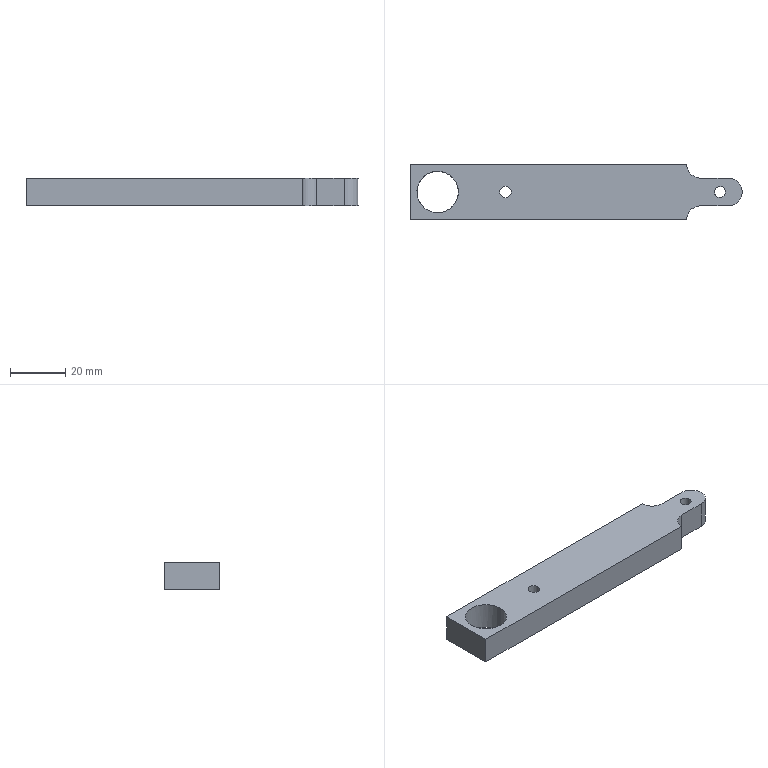Part | NX | features DATUM_CSYS 5, EXTRUDE 4, SKETCH 4, BLEND 2 | 1 solid | 13 faces | box 120 x 20 x 10 mm | volume 19969 mm3 | plane 7 | cylinder 6 | commonest cylinder face diameters 10 x3 4 x1 4.2 x1 15 x1
STEP:
#1=CARTESIAN_POINT('',(-60.,10.,0.));
#2=VERTEX_POINT('',#1);
#3=CARTESIAN_POINT('',(-60.,-10.,0.));
#4=VERTEX_POINT('',#3);
#5=CARTESIAN_POINT('',(-60.,10.,0.));
#6=DIRECTION('',(0.,-1.,0.));
#7=VECTOR('',#6,1000.);
#8=LINE('',#5,#7);
#9=EDGE_CURVE('',#2,#4,#8,.T.);
#10=ORIENTED_EDGE('',*,*,#9,.T.);
#11=CARTESIAN_POINT('',(-60.,-10.,10.));
#12=VERTEX_POINT('',#11);
#13=CARTESIAN_POINT('',(-60.,-10.,10.));
#14=DIRECTION('',(0.,0.,-1.));
#15=VECTOR('',#14,1000.);
#16=LINE('',#13,#15);
#17=EDGE_CURVE('',#12,#4,#16,.T.);
#18=ORIENTED_EDGE('',*,*,#17,.F.);
#19=CARTESIAN_POINT('',(-60.,10.,10.));
#20=VERTEX_POINT('',#19);
#21=CARTESIAN_POINT('',(-60.,10.,10.));
#22=DIRECTION('',(0.,-1.,0.));
#23=VECTOR('',#22,1000.);
#24=LINE('',#21,#23);
#25=EDGE_CURVE('',#20,#12,#24,.T.);
#26=ORIENTED_EDGE('',*,*,#25,.F.);
#27=CARTESIAN_POINT('',(-60.,10.,10.));
#28=DIRECTION('',(0.,0.,-1.));
#29=VECTOR('',#28,1000.);
#30=LINE('',#27,#29);
#31=EDGE_CURVE('',#20,#2,#30,.T.);
#32=ORIENTED_EDGE('',*,*,#31,.T.);
#33=EDGE_LOOP('',(#10,#18,#26,#32));
#34=FACE_BOUND('',#33,.T.);
#35=CARTESIAN_POINT('',(-60.,10.,10.));
#36=DIRECTION('',(1.,0.,0.));
#37=DIRECTION('',(0.,0.,-1.));
#38=AXIS2_PLACEMENT_3D('',#35,#36,#37);
#39=PLANE('',#38);
#40=ADVANCED_FACE('',(#34),#39,.F.);
#41=CARTESIAN_POINT('',(40.,-10.,0.));
#42=VERTEX_POINT('',#41);
#43=CARTESIAN_POINT('',(-60.,-10.,0.));
#44=DIRECTION('',(1.,0.,0.));
#45=VECTOR('',#44,1000.);
#46=LINE('',#43,#45);
#47=EDGE_CURVE('',#4,#42,#46,.T.);
#48=ORIENTED_EDGE('',*,*,#47,.T.);
#49=CARTESIAN_POINT('',(40.,-10.,10.));
#50=VERTEX_POINT('',#49);
#51=CARTESIAN_POINT('',(40.,-10.,10.));
#52=DIRECTION('',(0.,0.,1.));
#53=VECTOR('',#52,1000.);
#54=LINE('',#51,#53);
#55=EDGE_CURVE('',#42,#50,#54,.T.);
#56=ORIENTED_EDGE('',*,*,#55,.T.);
#57=CARTESIAN_POINT('',(-60.,-10.,10.));
#58=DIRECTION('',(1.,0.,0.));
#59=VECTOR('',#58,1000.);
#60=LINE('',#57,#59);
#61=EDGE_CURVE('',#12,#50,#60,.T.);
#62=ORIENTED_EDGE('',*,*,#61,.F.);
#63=ORIENTED_EDGE('',*,*,#17,.T.);
#64=EDGE_LOOP('',(#48,#56,#62,#63));
#65=FACE_BOUND('',#64,.T.);
#66=CARTESIAN_POINT('',(-60.,-10.,10.));
#67=DIRECTION('',(0.,1.,0.));
#68=DIRECTION('',(0.,0.,1.));
#69=AXIS2_PLACEMENT_3D('',#66,#67,#68);
#70=PLANE('',#69);
#71=ADVANCED_FACE('',(#65),#70,.F.);
#72=CARTESIAN_POINT('',(40.,10.,10.));
#73=VERTEX_POINT('',#72);
#74=CARTESIAN_POINT('',(60.,10.,10.));
#75=DIRECTION('',(-1.,0.,0.));
#76=VECTOR('',#75,1000.);
#77=LINE('',#74,#76);
#78=EDGE_CURVE('',#73,#20,#77,.T.);
#79=ORIENTED_EDGE('',*,*,#78,.F.);
#80=CARTESIAN_POINT('',(40.,10.,0.));
#81=VERTEX_POINT('',#80);
#82=CARTESIAN_POINT('',(40.,10.,10.));
#83=DIRECTION('',(0.,0.,-1.));
#84=VECTOR('',#83,1000.);
#85=LINE('',#82,#84);
#86=EDGE_CURVE('',#73,#81,#85,.T.);
#87=ORIENTED_EDGE('',*,*,#86,.T.);
#88=CARTESIAN_POINT('',(60.,10.,0.));
#89=DIRECTION('',(-1.,0.,0.));
#90=VECTOR('',#89,1000.);
#91=LINE('',#88,#90);
#92=EDGE_CURVE('',#81,#2,#91,.T.);
#93=ORIENTED_EDGE('',*,*,#92,.T.);
#94=ORIENTED_EDGE('',*,*,#31,.F.);
#95=EDGE_LOOP('',(#79,#87,#93,#94));
#96=FACE_BOUND('',#95,.T.);
#97=CARTESIAN_POINT('',(60.,10.,10.));
#98=DIRECTION('',(0.,-1.,0.));
#99=DIRECTION('',(0.,0.,-1.));
#100=AXIS2_PLACEMENT_3D('',#97,#98,#99);
#101=PLANE('',#100);
#102=ADVANCED_FACE('',(#96),#101,.F.);
#103=CARTESIAN_POINT('',(-23.4,0.,10.));
#104=VERTEX_POINT('',#103);
#105=CARTESIAN_POINT('',(-25.5,0.,10.));
#106=DIRECTION('',(0.,0.,1.));
#107=DIRECTION('',(1.,0.,0.));
#108=AXIS2_PLACEMENT_3D('',#105,#106,#107);
#109=CIRCLE('',#108,2.1);
#110=EDGE_CURVE('',#104,#104,#109,.T.);
#111=ORIENTED_EDGE('',*,*,#110,.F.);
#112=EDGE_LOOP('',(#111));
#113=FACE_BOUND('',#112,.T.);
#114=CARTESIAN_POINT('',(55.,-5.,10.));
#115=VERTEX_POINT('',#114);
#116=CARTESIAN_POINT('',(45.,-5.,10.));
#117=VERTEX_POINT('',#116);
#118=CARTESIAN_POINT('',(126.735,-5.,10.));
#119=DIRECTION('',(-1.,0.,0.));
#120=VECTOR('',#119,1000.);
#121=LINE('',#118,#120);
#122=EDGE_CURVE('',#115,#117,#121,.T.);
#123=ORIENTED_EDGE('',*,*,#122,.F.);
#124=CARTESIAN_POINT('',(55.,5.,10.));
#125=VERTEX_POINT('',#124);
#126=CARTESIAN_POINT('',(55.,0.,10.));
#127=DIRECTION('',(0.,0.,1.));
#128=DIRECTION('',(1.,0.,0.));
#129=AXIS2_PLACEMENT_3D('',#126,#127,#128);
#130=CIRCLE('',#129,5.);
#131=EDGE_CURVE('',#115,#125,#130,.T.);
#132=ORIENTED_EDGE('',*,*,#131,.T.);
#133=CARTESIAN_POINT('',(45.,5.,10.));
#134=VERTEX_POINT('',#133);
#135=CARTESIAN_POINT('',(40.,5.,10.));
#136=DIRECTION('',(1.,0.,0.));
#137=VECTOR('',#136,1000.);
#138=LINE('',#135,#137);
#139=EDGE_CURVE('',#134,#125,#138,.T.);
#140=ORIENTED_EDGE('',*,*,#139,.F.);
#141=CARTESIAN_POINT('',(45.,10.,10.));
#142=DIRECTION('',(0.,0.,1.));
#143=DIRECTION('',(1.,0.,0.));
#144=AXIS2_PLACEMENT_3D('',#141,#142,#143);
#145=CIRCLE('',#144,5.);
#146=EDGE_CURVE('',#134,#73,#145,.F.);
#147=ORIENTED_EDGE('',*,*,#146,.T.);
#148=ORIENTED_EDGE('',*,*,#78,.T.);
#149=ORIENTED_EDGE('',*,*,#25,.T.);
#150=ORIENTED_EDGE('',*,*,#61,.T.);
#151=CARTESIAN_POINT('',(45.,-10.,10.));
#152=DIRECTION('',(0.,0.,1.));
#153=DIRECTION('',(1.,0.,0.));
#154=AXIS2_PLACEMENT_3D('',#151,#152,#153);
#155=CIRCLE('',#154,5.);
#156=EDGE_CURVE('',#50,#117,#155,.F.);
#157=ORIENTED_EDGE('',*,*,#156,.T.);
#158=EDGE_LOOP('',(#123,#132,#140,#147,#148,#149,#150,#157));
#159=FACE_BOUND('',#158,.T.);
#160=CARTESIAN_POINT('',(52.,2.,10.));
#161=VERTEX_POINT('',#160);
#162=CARTESIAN_POINT('',(52.,0.,10.));
#163=DIRECTION('',(0.,0.,1.));
#164=DIRECTION('',(0.,1.,0.));
#165=AXIS2_PLACEMENT_3D('',#162,#163,#164);
#166=CIRCLE('',#165,2.);
#167=EDGE_CURVE('',#161,#161,#166,.T.);
#168=ORIENTED_EDGE('',*,*,#167,.F.);
#169=EDGE_LOOP('',(#168));
#170=FACE_BOUND('',#169,.T.);
#171=CARTESIAN_POINT('',(-50.,7.5,10.));
#172=VERTEX_POINT('',#171);
#173=CARTESIAN_POINT('',(-50.,0.,10.));
#174=DIRECTION('',(0.,0.,1.));
#175=DIRECTION('',(0.,1.,0.));
#176=AXIS2_PLACEMENT_3D('',#173,#174,#175);
#177=CIRCLE('',#176,7.5);
#178=EDGE_CURVE('',#172,#172,#177,.T.);
#179=ORIENTED_EDGE('',*,*,#178,.F.);
#180=EDGE_LOOP('',(#179));
#181=FACE_BOUND('',#180,.T.);
#182=CARTESIAN_POINT('',(0.,0.,10.));
#183=DIRECTION('',(0.,0.,1.));
#184=DIRECTION('',(1.,0.,0.));
#185=AXIS2_PLACEMENT_3D('',#182,#183,#184);
#186=PLANE('',#185);
#187=ADVANCED_FACE('',(#113,#159,#170,#181),#186,.T.);
#188=CARTESIAN_POINT('',(-23.4,0.,0.));
#189=VERTEX_POINT('',#188);
#190=CARTESIAN_POINT('',(-25.5,0.,0.));
#191=DIRECTION('',(0.,0.,1.));
#192=DIRECTION('',(1.,0.,0.));
#193=AXIS2_PLACEMENT_3D('',#190,#191,#192);
#194=CIRCLE('',#193,2.1);
#195=EDGE_CURVE('',#189,#189,#194,.T.);
#196=ORIENTED_EDGE('',*,*,#195,.T.);
#197=EDGE_LOOP('',(#196));
#198=FACE_BOUND('',#197,.T.);
#199=CARTESIAN_POINT('',(54.,0.,0.));
#200=VERTEX_POINT('',#199);
#201=CARTESIAN_POINT('',(52.,0.,0.));
#202=DIRECTION('',(0.,0.,1.));
#203=DIRECTION('',(1.,0.,0.));
#204=AXIS2_PLACEMENT_3D('',#201,#202,#203);
#205=CIRCLE('',#204,2.);
#206=EDGE_CURVE('',#200,#200,#205,.T.);
#207=ORIENTED_EDGE('',*,*,#206,.T.);
#208=EDGE_LOOP('',(#207));
#209=FACE_BOUND('',#208,.T.);
#210=CARTESIAN_POINT('',(-42.5,0.,0.));
#211=VERTEX_POINT('',#210);
#212=CARTESIAN_POINT('',(-50.,0.,0.));
#213=DIRECTION('',(0.,0.,1.));
#214=DIRECTION('',(1.,0.,0.));
#215=AXIS2_PLACEMENT_3D('',#212,#213,#214);
#216=CIRCLE('',#215,7.5);
#217=EDGE_CURVE('',#211,#211,#216,.T.);
#218=ORIENTED_EDGE('',*,*,#217,.T.);
#219=EDGE_LOOP('',(#218));
#220=FACE_BOUND('',#219,.T.);
#221=CARTESIAN_POINT('',(55.,5.,0.));
#222=VERTEX_POINT('',#221);
#223=CARTESIAN_POINT('',(55.,-5.,0.));
#224=VERTEX_POINT('',#223);
#225=CARTESIAN_POINT('',(55.,0.,0.));
#226=DIRECTION('',(0.,0.,1.));
#227=DIRECTION('',(1.,0.,0.));
#228=AXIS2_PLACEMENT_3D('',#225,#226,#227);
#229=CIRCLE('',#228,5.);
#230=EDGE_CURVE('',#222,#224,#229,.F.);
#231=ORIENTED_EDGE('',*,*,#230,.T.);
#232=CARTESIAN_POINT('',(45.,-5.,0.));
#233=VERTEX_POINT('',#232);
#234=CARTESIAN_POINT('',(0.,-5.,0.));
#235=DIRECTION('',(-1.,0.,0.));
#236=VECTOR('',#235,1000.);
#237=LINE('',#234,#236);
#238=EDGE_CURVE('',#224,#233,#237,.T.);
#239=ORIENTED_EDGE('',*,*,#238,.T.);
#240=CARTESIAN_POINT('',(45.,-10.,0.));
#241=DIRECTION('',(0.,0.,1.));
#242=DIRECTION('',(1.,0.,0.));
#243=AXIS2_PLACEMENT_3D('',#240,#241,#242);
#244=CIRCLE('',#243,5.);
#245=EDGE_CURVE('',#233,#42,#244,.T.);
#246=ORIENTED_EDGE('',*,*,#245,.T.);
#247=ORIENTED_EDGE('',*,*,#47,.F.);
#248=ORIENTED_EDGE('',*,*,#9,.F.);
#249=ORIENTED_EDGE('',*,*,#92,.F.);
#250=CARTESIAN_POINT('',(45.,5.,0.));
#251=VERTEX_POINT('',#250);
#252=CARTESIAN_POINT('',(45.,10.,0.));
#253=DIRECTION('',(0.,0.,1.));
#254=DIRECTION('',(1.,0.,0.));
#255=AXIS2_PLACEMENT_3D('',#252,#253,#254);
#256=CIRCLE('',#255,5.);
#257=EDGE_CURVE('',#81,#251,#256,.T.);
#258=ORIENTED_EDGE('',*,*,#257,.T.);
#259=CARTESIAN_POINT('',(0.,5.,0.));
#260=DIRECTION('',(1.,0.,0.));
#261=VECTOR('',#260,1000.);
#262=LINE('',#259,#261);
#263=EDGE_CURVE('',#251,#222,#262,.T.);
#264=ORIENTED_EDGE('',*,*,#263,.T.);
#265=EDGE_LOOP('',(#231,#239,#246,#247,#248,#249,#258,#264));
#266=FACE_BOUND('',#265,.T.);
#267=CARTESIAN_POINT('',(0.,0.,0.));
#268=DIRECTION('',(0.,0.,1.));
#269=DIRECTION('',(1.,0.,0.));
#270=AXIS2_PLACEMENT_3D('',#267,#268,#269);
#271=PLANE('',#270);
#272=ADVANCED_FACE('',(#198,#209,#220,#266),#271,.F.);
#273=ORIENTED_EDGE('',*,*,#178,.T.);
#274=EDGE_LOOP('',(#273));
#275=FACE_BOUND('',#274,.T.);
#276=ORIENTED_EDGE('',*,*,#217,.F.);
#277=EDGE_LOOP('',(#276));
#278=FACE_BOUND('',#277,.T.);
#279=CARTESIAN_POINT('',(-50.,0.,-5.));
#280=DIRECTION('',(0.,0.,1.));
#281=DIRECTION('',(1.,0.,0.));
#282=AXIS2_PLACEMENT_3D('',#279,#280,#281);
#283=CYLINDRICAL_SURFACE('',#282,7.5);
#284=ADVANCED_FACE('',(#275,#278),#283,.F.);
#285=ORIENTED_EDGE('',*,*,#167,.T.);
#286=EDGE_LOOP('',(#285));
#287=FACE_BOUND('',#286,.T.);
#288=ORIENTED_EDGE('',*,*,#206,.F.);
#289=EDGE_LOOP('',(#288));
#290=FACE_BOUND('',#289,.T.);
#291=CARTESIAN_POINT('',(52.,0.,-5.));
#292=DIRECTION('',(0.,0.,1.));
#293=DIRECTION('',(1.,0.,0.));
#294=AXIS2_PLACEMENT_3D('',#291,#292,#293);
#295=CYLINDRICAL_SURFACE('',#294,2.);
#296=ADVANCED_FACE('',(#287,#290),#295,.F.);
#297=ORIENTED_EDGE('',*,*,#238,.F.);
#298=CARTESIAN_POINT('',(55.,-5.,-10.));
#299=DIRECTION('',(0.,0.,-1.));
#300=VECTOR('',#299,1000.);
#301=LINE('',#298,#300);
#302=EDGE_CURVE('',#224,#115,#301,.F.);
#303=ORIENTED_EDGE('',*,*,#302,.T.);
#304=ORIENTED_EDGE('',*,*,#122,.T.);
#305=CARTESIAN_POINT('',(45.,-5.,0.));
#306=DIRECTION('',(0.,0.,-1.));
#307=VECTOR('',#306,1000.);
#308=LINE('',#305,#307);
#309=EDGE_CURVE('',#117,#233,#308,.T.);
#310=ORIENTED_EDGE('',*,*,#309,.T.);
#311=EDGE_LOOP('',(#297,#303,#304,#310));
#312=FACE_BOUND('',#311,.T.);
#313=CARTESIAN_POINT('',(126.735,-5.,-10.));
#314=DIRECTION('',(0.,1.,0.));
#315=DIRECTION('',(-1.,0.,0.));
#316=AXIS2_PLACEMENT_3D('',#313,#314,#315);
#317=PLANE('',#316);
#318=ADVANCED_FACE('',(#312),#317,.F.);
#319=ORIENTED_EDGE('',*,*,#139,.T.);
#320=CARTESIAN_POINT('',(55.,5.,-10.));
#321=DIRECTION('',(0.,0.,1.));
#322=VECTOR('',#321,1000.);
#323=LINE('',#320,#322);
#324=EDGE_CURVE('',#125,#222,#323,.F.);
#325=ORIENTED_EDGE('',*,*,#324,.T.);
#326=ORIENTED_EDGE('',*,*,#263,.F.);
#327=CARTESIAN_POINT('',(45.,5.,10.));
#328=DIRECTION('',(0.,0.,-1.));
#329=VECTOR('',#328,1000.);
#330=LINE('',#327,#329);
#331=EDGE_CURVE('',#251,#134,#330,.F.);
#332=ORIENTED_EDGE('',*,*,#331,.T.);
#333=EDGE_LOOP('',(#319,#325,#326,#332));
#334=FACE_BOUND('',#333,.T.);
#335=CARTESIAN_POINT('',(40.,5.,-10.));
#336=DIRECTION('',(0.,-1.,0.));
#337=DIRECTION('',(1.,0.,0.));
#338=AXIS2_PLACEMENT_3D('',#335,#336,#337);
#339=PLANE('',#338);
#340=ADVANCED_FACE('',(#334),#339,.F.);
#341=ORIENTED_EDGE('',*,*,#146,.F.);
#342=ORIENTED_EDGE('',*,*,#331,.F.);
#343=ORIENTED_EDGE('',*,*,#257,.F.);
#344=ORIENTED_EDGE('',*,*,#86,.F.);
#345=EDGE_LOOP('',(#341,#342,#343,#344));
#346=FACE_BOUND('',#345,.T.);
#347=CARTESIAN_POINT('',(45.,10.,-10.));
#348=DIRECTION('',(0.,0.,1.));
#349=DIRECTION('',(1.,0.,0.));
#350=AXIS2_PLACEMENT_3D('',#347,#348,#349);
#351=CYLINDRICAL_SURFACE('',#350,5.);
#352=ADVANCED_FACE('',(#346),#351,.F.);
#353=ORIENTED_EDGE('',*,*,#156,.F.);
#354=ORIENTED_EDGE('',*,*,#55,.F.);
#355=ORIENTED_EDGE('',*,*,#245,.F.);
#356=ORIENTED_EDGE('',*,*,#309,.F.);
#357=EDGE_LOOP('',(#353,#354,#355,#356));
#358=FACE_BOUND('',#357,.T.);
#359=CARTESIAN_POINT('',(45.,-10.,-10.));
#360=DIRECTION('',(0.,0.,1.));
#361=DIRECTION('',(1.,0.,0.));
#362=AXIS2_PLACEMENT_3D('',#359,#360,#361);
#363=CYLINDRICAL_SURFACE('',#362,5.);
#364=ADVANCED_FACE('',(#358),#363,.F.);
#365=ORIENTED_EDGE('',*,*,#324,.F.);
#366=ORIENTED_EDGE('',*,*,#131,.F.);
#367=ORIENTED_EDGE('',*,*,#302,.F.);
#368=ORIENTED_EDGE('',*,*,#230,.F.);
#369=EDGE_LOOP('',(#365,#366,#367,#368));
#370=FACE_BOUND('',#369,.T.);
#371=CARTESIAN_POINT('',(55.,0.,10.));
#372=DIRECTION('',(0.,0.,1.));
#373=DIRECTION('',(1.,0.,0.));
#374=AXIS2_PLACEMENT_3D('',#371,#372,#373);
#375=CYLINDRICAL_SURFACE('',#374,5.);
#376=ADVANCED_FACE('',(#370),#375,.T.);
#377=ORIENTED_EDGE('',*,*,#110,.T.);
#378=EDGE_LOOP('',(#377));
#379=FACE_BOUND('',#378,.T.);
#380=ORIENTED_EDGE('',*,*,#195,.F.);
#381=EDGE_LOOP('',(#380));
#382=FACE_BOUND('',#381,.T.);
#383=CARTESIAN_POINT('',(-25.5,0.,-10.));
#384=DIRECTION('',(0.,0.,1.));
#385=DIRECTION('',(1.,0.,0.));
#386=AXIS2_PLACEMENT_3D('',#383,#384,#385);
#387=CYLINDRICAL_SURFACE('',#386,2.1);
#388=ADVANCED_FACE('',(#379,#382),#387,.F.);
#389=CLOSED_SHELL('',(#40,#71,#102,#187,#272,#284,#296,#318,#340,#352,#364,#376,#388));
#390=MANIFOLD_SOLID_BREP('',#389);
#391=(LENGTH_UNIT()NAMED_UNIT(*)SI_UNIT(.MILLI.,.METRE.));
#392=UNCERTAINTY_MEASURE_WITH_UNIT(LENGTH_MEASURE(0.00001),#391,'','');
#393=(NAMED_UNIT(*)PLANE_ANGLE_UNIT()SI_UNIT($,.RADIAN.));
#394=(NAMED_UNIT(*)SI_UNIT($,.STERADIAN.)SOLID_ANGLE_UNIT());
#395=(GEOMETRIC_REPRESENTATION_CONTEXT(3)GLOBAL_UNCERTAINTY_ASSIGNED_CONTEXT((#392))GLOBAL_UNIT_ASSIGNED_CONTEXT((#391,#393,#394))REPRESENTATION_CONTEXT('',''));
#396=ADVANCED_BREP_SHAPE_REPRESENTATION('',(#390),#395);